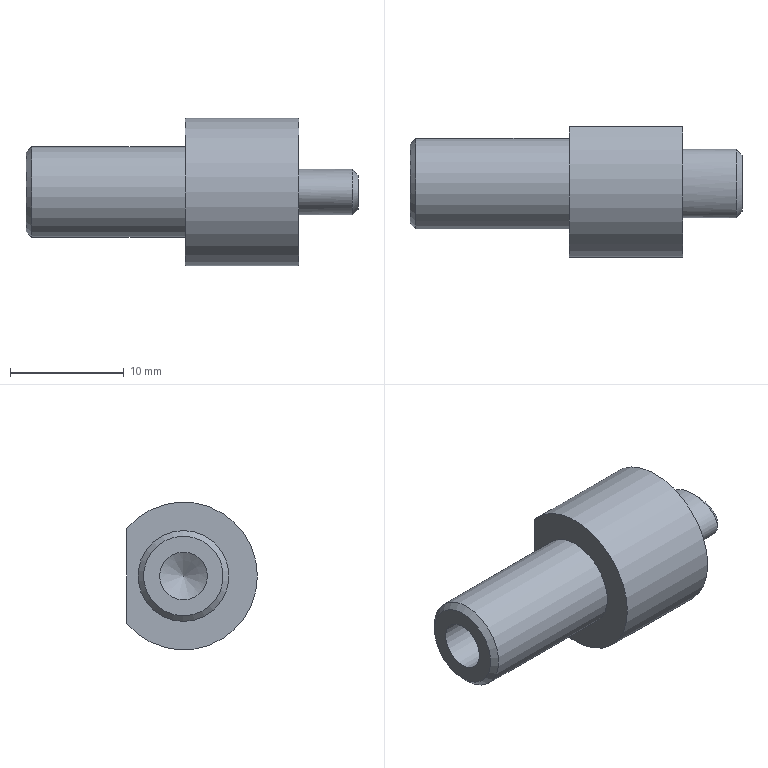Part | NX | features BREP 1 | 1 solid | 12 faces | box 29.2 x 11.5 x 13 mm | volume 1862 mm3 | plane 5 | cylinder 3 | spline 2 | cone 2 | commonest cylinder face diameters 4.2 x1 8 x1 13 x1